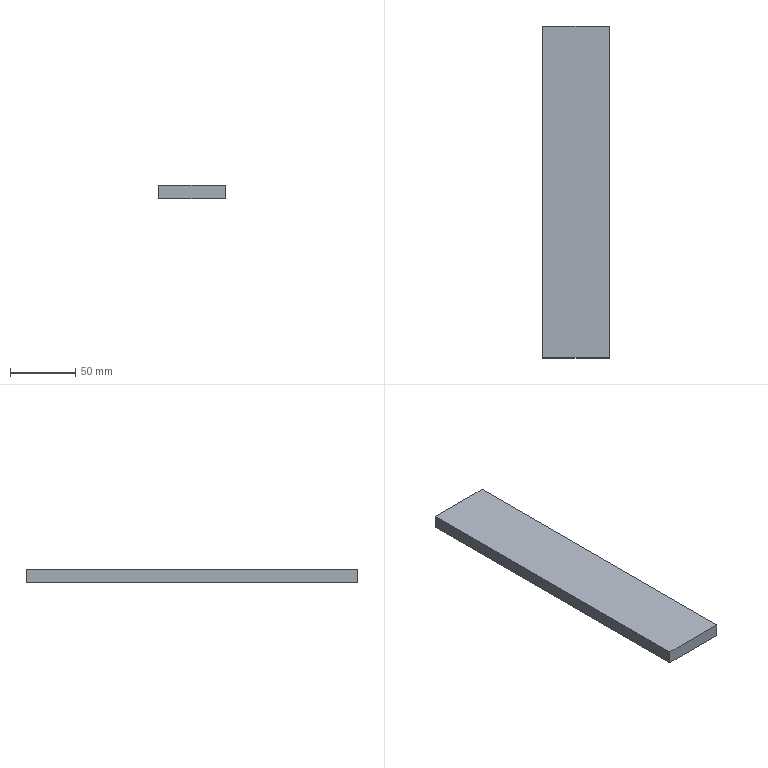Part | SolidWorks | features Extrusion 1 | 1 solid | 6 faces | box 50.8 x 254 x 10 mm | volume 129032 mm3 | plane 6
STEP:
#1=CARTESIAN_POINT('',(-25.4,127.,-5.));
#2=VERTEX_POINT('',#1);
#3=CARTESIAN_POINT('',(-25.4,-127.,-5.));
#4=VERTEX_POINT('',#3);
#5=CARTESIAN_POINT('',(-25.4,127.,-5.));
#6=DIRECTION('',(0.,-1.,0.));
#7=VECTOR('',#6,1000.);
#8=LINE('',#5,#7);
#9=EDGE_CURVE('',#2,#4,#8,.T.);
#10=ORIENTED_EDGE('',*,*,#9,.T.);
#11=CARTESIAN_POINT('',(-25.4,-127.,5.));
#12=VERTEX_POINT('',#11);
#13=CARTESIAN_POINT('',(-25.4,-127.,5.));
#14=DIRECTION('',(0.,0.,-1.));
#15=VECTOR('',#14,1000.);
#16=LINE('',#13,#15);
#17=EDGE_CURVE('',#12,#4,#16,.T.);
#18=ORIENTED_EDGE('',*,*,#17,.F.);
#19=CARTESIAN_POINT('',(-25.4,127.,5.));
#20=VERTEX_POINT('',#19);
#21=CARTESIAN_POINT('',(-25.4,127.,5.));
#22=DIRECTION('',(0.,-1.,0.));
#23=VECTOR('',#22,1000.);
#24=LINE('',#21,#23);
#25=EDGE_CURVE('',#20,#12,#24,.T.);
#26=ORIENTED_EDGE('',*,*,#25,.F.);
#27=CARTESIAN_POINT('',(-25.4,127.,5.));
#28=DIRECTION('',(0.,0.,-1.));
#29=VECTOR('',#28,1000.);
#30=LINE('',#27,#29);
#31=EDGE_CURVE('',#20,#2,#30,.T.);
#32=ORIENTED_EDGE('',*,*,#31,.T.);
#33=EDGE_LOOP('',(#10,#18,#26,#32));
#34=FACE_OUTER_BOUND('',#33,.T.);
#35=CARTESIAN_POINT('',(-25.4,127.,5.));
#36=DIRECTION('',(1.,0.,0.));
#37=DIRECTION('',(0.,1.,0.));
#38=AXIS2_PLACEMENT_3D('',#35,#36,#37);
#39=PLANE('',#38);
#40=ADVANCED_FACE('',(#34),#39,.F.);
#41=CARTESIAN_POINT('',(25.4,-127.,-5.));
#42=VERTEX_POINT('',#41);
#43=CARTESIAN_POINT('',(-25.4,-127.,-5.));
#44=DIRECTION('',(1.,0.,0.));
#45=VECTOR('',#44,1000.);
#46=LINE('',#43,#45);
#47=EDGE_CURVE('',#4,#42,#46,.T.);
#48=ORIENTED_EDGE('',*,*,#47,.T.);
#49=CARTESIAN_POINT('',(25.4,-127.,5.));
#50=VERTEX_POINT('',#49);
#51=CARTESIAN_POINT('',(25.4,-127.,5.));
#52=DIRECTION('',(0.,0.,-1.));
#53=VECTOR('',#52,1000.);
#54=LINE('',#51,#53);
#55=EDGE_CURVE('',#50,#42,#54,.T.);
#56=ORIENTED_EDGE('',*,*,#55,.F.);
#57=CARTESIAN_POINT('',(-25.4,-127.,5.));
#58=DIRECTION('',(1.,0.,0.));
#59=VECTOR('',#58,1000.);
#60=LINE('',#57,#59);
#61=EDGE_CURVE('',#12,#50,#60,.T.);
#62=ORIENTED_EDGE('',*,*,#61,.F.);
#63=ORIENTED_EDGE('',*,*,#17,.T.);
#64=EDGE_LOOP('',(#48,#56,#62,#63));
#65=FACE_OUTER_BOUND('',#64,.T.);
#66=CARTESIAN_POINT('',(-25.4,-127.,5.));
#67=DIRECTION('',(0.,1.,0.));
#68=DIRECTION('',(0.,0.,1.));
#69=AXIS2_PLACEMENT_3D('',#66,#67,#68);
#70=PLANE('',#69);
#71=ADVANCED_FACE('',(#65),#70,.F.);
#72=CARTESIAN_POINT('',(25.4,127.,-5.));
#73=VERTEX_POINT('',#72);
#74=CARTESIAN_POINT('',(25.4,127.,-5.));
#75=DIRECTION('',(0.,1.,0.));
#76=VECTOR('',#75,1000.);
#77=LINE('',#74,#76);
#78=EDGE_CURVE('',#42,#73,#77,.T.);
#79=ORIENTED_EDGE('',*,*,#78,.T.);
#80=CARTESIAN_POINT('',(25.4,127.,5.));
#81=VERTEX_POINT('',#80);
#82=CARTESIAN_POINT('',(25.4,127.,5.));
#83=DIRECTION('',(0.,0.,-1.));
#84=VECTOR('',#83,1000.);
#85=LINE('',#82,#84);
#86=EDGE_CURVE('',#81,#73,#85,.T.);
#87=ORIENTED_EDGE('',*,*,#86,.F.);
#88=CARTESIAN_POINT('',(25.4,127.,5.));
#89=DIRECTION('',(0.,1.,0.));
#90=VECTOR('',#89,1000.);
#91=LINE('',#88,#90);
#92=EDGE_CURVE('',#50,#81,#91,.T.);
#93=ORIENTED_EDGE('',*,*,#92,.F.);
#94=ORIENTED_EDGE('',*,*,#55,.T.);
#95=EDGE_LOOP('',(#79,#87,#93,#94));
#96=FACE_OUTER_BOUND('',#95,.T.);
#97=CARTESIAN_POINT('',(25.4,127.,5.));
#98=DIRECTION('',(-1.,0.,0.));
#99=DIRECTION('',(0.,-1.,0.));
#100=AXIS2_PLACEMENT_3D('',#97,#98,#99);
#101=PLANE('',#100);
#102=ADVANCED_FACE('',(#96),#101,.F.);
#103=CARTESIAN_POINT('',(-25.4,127.,-5.));
#104=DIRECTION('',(-1.,0.,0.));
#105=VECTOR('',#104,1000.);
#106=LINE('',#103,#105);
#107=EDGE_CURVE('',#73,#2,#106,.T.);
#108=ORIENTED_EDGE('',*,*,#107,.T.);
#109=ORIENTED_EDGE('',*,*,#31,.F.);
#110=CARTESIAN_POINT('',(-25.4,127.,5.));
#111=DIRECTION('',(-1.,0.,0.));
#112=VECTOR('',#111,1000.);
#113=LINE('',#110,#112);
#114=EDGE_CURVE('',#81,#20,#113,.T.);
#115=ORIENTED_EDGE('',*,*,#114,.F.);
#116=ORIENTED_EDGE('',*,*,#86,.T.);
#117=EDGE_LOOP('',(#108,#109,#115,#116));
#118=FACE_OUTER_BOUND('',#117,.T.);
#119=CARTESIAN_POINT('',(-25.4,127.,5.));
#120=DIRECTION('',(0.,-1.,0.));
#121=DIRECTION('',(0.,0.,-1.));
#122=AXIS2_PLACEMENT_3D('',#119,#120,#121);
#123=PLANE('',#122);
#124=ADVANCED_FACE('',(#118),#123,.F.);
#125=ORIENTED_EDGE('',*,*,#25,.T.);
#126=ORIENTED_EDGE('',*,*,#61,.T.);
#127=ORIENTED_EDGE('',*,*,#92,.T.);
#128=ORIENTED_EDGE('',*,*,#114,.T.);
#129=EDGE_LOOP('',(#125,#126,#127,#128));
#130=FACE_OUTER_BOUND('',#129,.T.);
#131=CARTESIAN_POINT('',(0.,0.,5.));
#132=DIRECTION('',(0.,0.,1.));
#133=DIRECTION('',(1.,0.,0.));
#134=AXIS2_PLACEMENT_3D('',#131,#132,#133);
#135=PLANE('',#134);
#136=ADVANCED_FACE('',(#130),#135,.T.);
#137=ORIENTED_EDGE('',*,*,#9,.F.);
#138=ORIENTED_EDGE('',*,*,#107,.F.);
#139=ORIENTED_EDGE('',*,*,#78,.F.);
#140=ORIENTED_EDGE('',*,*,#47,.F.);
#141=EDGE_LOOP('',(#137,#138,#139,#140));
#142=FACE_OUTER_BOUND('',#141,.T.);
#143=CARTESIAN_POINT('',(0.,0.,-5.));
#144=DIRECTION('',(0.,0.,1.));
#145=DIRECTION('',(1.,0.,0.));
#146=AXIS2_PLACEMENT_3D('',#143,#144,#145);
#147=PLANE('',#146);
#148=ADVANCED_FACE('',(#142),#147,.F.);
#149=CLOSED_SHELL('',(#40,#71,#102,#124,#136,#148));
#150=MANIFOLD_SOLID_BREP('',#149);
#151=CARTESIAN_POINT('',(0.,0.,0.));
#152=DIRECTION('',(0.,0.,1.));
#153=DIRECTION('',(1.,0.,0.));
#154=AXIS2_PLACEMENT_3D('',#151,#152,#153);
#155=(LENGTH_UNIT()NAMED_UNIT(*)SI_UNIT(.MILLI.,.METRE.));
#156=UNCERTAINTY_MEASURE_WITH_UNIT(LENGTH_MEASURE(0.00001),#155,'','');
#157=(NAMED_UNIT(*)PLANE_ANGLE_UNIT()SI_UNIT($,.RADIAN.));
#158=(NAMED_UNIT(*)SI_UNIT($,.STERADIAN.)SOLID_ANGLE_UNIT());
#159=(GEOMETRIC_REPRESENTATION_CONTEXT(3)GLOBAL_UNCERTAINTY_ASSIGNED_CONTEXT((#156))GLOBAL_UNIT_ASSIGNED_CONTEXT((#155,#157,#158))REPRESENTATION_CONTEXT('',''));
#160=ADVANCED_BREP_SHAPE_REPRESENTATION('',(#150,#154),#159);